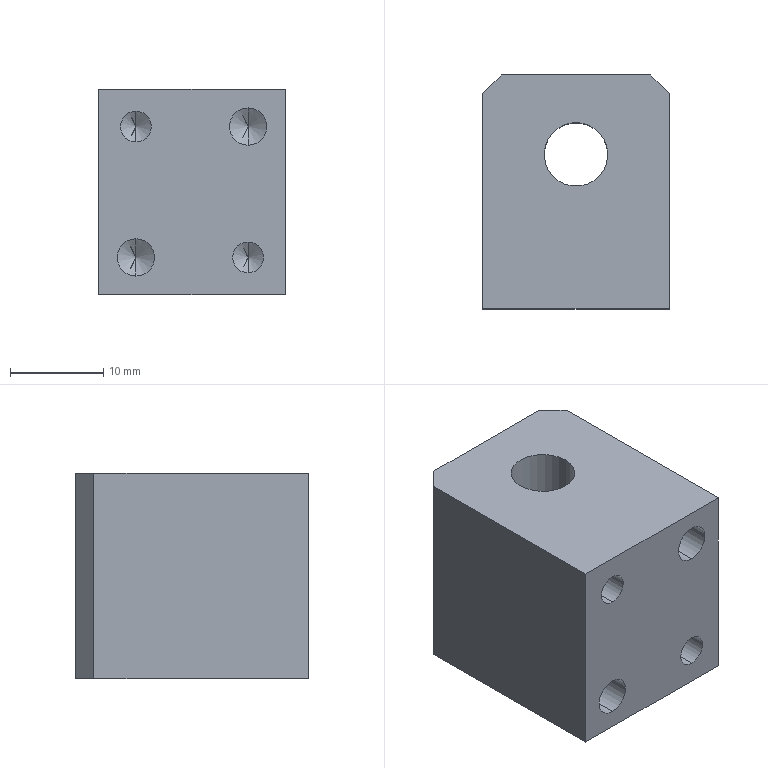Part | SolidWorks | features HoleWzd 3, Chamfer 1, Extrusion 1 | 1 solid | 26 faces | box 20 x 25 x 22 mm | volume 9700 mm3 | cylinder 10 | cone 8 | plane 8 | commonest cylinder face diameters 3.3 x4 4 x4 6.8 x2
STEP:
#1=CARTESIAN_POINT('',(6.,-4.5,9.));
#2=VERTEX_POINT('',#1);
#3=CARTESIAN_POINT('',(6.,-4.5,5.));
#4=VERTEX_POINT('',#3);
#5=CARTESIAN_POINT('',(6.,-4.5,7.));
#6=DIRECTION('',(0.,-1.,0.));
#7=DIRECTION('',(0.,0.,-1.));
#8=AXIS2_PLACEMENT_3D('',#5,#6,#7);
#9=CIRCLE('',#8,2.);
#10=EDGE_CURVE('',#2,#4,#9,.T.);
#11=ORIENTED_EDGE('',*,*,#10,.F.);
#12=CARTESIAN_POINT('',(6.,-12.5,9.));
#13=VERTEX_POINT('',#12);
#14=CARTESIAN_POINT('',(6.,-12.5,9.));
#15=DIRECTION('',(0.,-1.,0.));
#16=VECTOR('',#15,1000.);
#17=LINE('',#14,#16);
#18=EDGE_CURVE('',#2,#13,#17,.T.);
#19=ORIENTED_EDGE('',*,*,#18,.T.);
#20=CARTESIAN_POINT('',(6.,-12.5,5.));
#21=VERTEX_POINT('',#20);
#22=CARTESIAN_POINT('',(6.,-12.5,7.));
#23=DIRECTION('',(0.,-1.,0.));
#24=DIRECTION('',(0.,0.,-1.));
#25=AXIS2_PLACEMENT_3D('',#22,#23,#24);
#26=CIRCLE('',#25,2.);
#27=EDGE_CURVE('',#13,#21,#26,.T.);
#28=ORIENTED_EDGE('',*,*,#27,.T.);
#29=CARTESIAN_POINT('',(6.,-12.5,5.));
#30=DIRECTION('',(0.,-1.,0.));
#31=VECTOR('',#30,1000.);
#32=LINE('',#29,#31);
#33=EDGE_CURVE('',#4,#21,#32,.T.);
#34=ORIENTED_EDGE('',*,*,#33,.F.);
#35=EDGE_LOOP('',(#11,#19,#28,#34));
#36=FACE_OUTER_BOUND('',#35,.T.);
#37=CARTESIAN_POINT('',(6.,-12.5,7.));
#38=DIRECTION('',(0.,-1.,0.));
#39=DIRECTION('',(0.,0.,-1.));
#40=AXIS2_PLACEMENT_3D('',#37,#38,#39);
#41=CYLINDRICAL_SURFACE('',#40,2.);
#42=ADVANCED_FACE('',(#36),#41,.F.);
#43=CARTESIAN_POINT('',(6.,-3.298,7.));
#44=VERTEX_POINT('',#43);
#45=CARTESIAN_POINT('',(6.,-4.5,5.));
#46=DIRECTION('',(0.,-0.515,-0.8572));
#47=VECTOR('',#46,1000.);
#48=LINE('',#45,#47);
#49=EDGE_CURVE('',#44,#4,#48,.T.);
#50=ORIENTED_EDGE('',*,*,#49,.F.);
#51=CARTESIAN_POINT('',(6.,-4.5,9.));
#52=DIRECTION('',(0.,-0.515,0.8572));
#53=VECTOR('',#52,1000.);
#54=LINE('',#51,#53);
#55=EDGE_CURVE('',#44,#2,#54,.T.);
#56=ORIENTED_EDGE('',*,*,#55,.T.);
#57=ORIENTED_EDGE('',*,*,#10,.T.);
#58=EDGE_LOOP('',(#50,#56,#57));
#59=FACE_OUTER_BOUND('',#58,.T.);
#60=CARTESIAN_POINT('',(6.,-4.5,7.));
#61=DIRECTION('',(0.,-1.,0.));
#62=DIRECTION('',(0.,0.,-1.));
#63=AXIS2_PLACEMENT_3D('',#60,#61,#62);
#64=CONICAL_SURFACE('',#63,2.,1.03);
#65=ADVANCED_FACE('',(#59),#64,.F.);
#66=CARTESIAN_POINT('',(-6.,-4.5,-5.));
#67=VERTEX_POINT('',#66);
#68=CARTESIAN_POINT('',(-6.,-4.5,-9.));
#69=VERTEX_POINT('',#68);
#70=CARTESIAN_POINT('',(-6.,-4.5,-7.));
#71=DIRECTION('',(0.,-1.,0.));
#72=DIRECTION('',(0.,0.,-1.));
#73=AXIS2_PLACEMENT_3D('',#70,#71,#72);
#74=CIRCLE('',#73,2.);
#75=EDGE_CURVE('',#67,#69,#74,.T.);
#76=ORIENTED_EDGE('',*,*,#75,.F.);
#77=CARTESIAN_POINT('',(-6.,-12.5,-5.));
#78=VERTEX_POINT('',#77);
#79=CARTESIAN_POINT('',(-6.,-12.5,-5.));
#80=DIRECTION('',(0.,-1.,0.));
#81=VECTOR('',#80,1000.);
#82=LINE('',#79,#81);
#83=EDGE_CURVE('',#67,#78,#82,.T.);
#84=ORIENTED_EDGE('',*,*,#83,.T.);
#85=CARTESIAN_POINT('',(-6.,-12.5,-9.));
#86=VERTEX_POINT('',#85);
#87=CARTESIAN_POINT('',(-6.,-12.5,-7.));
#88=DIRECTION('',(0.,-1.,0.));
#89=DIRECTION('',(0.,0.,-1.));
#90=AXIS2_PLACEMENT_3D('',#87,#88,#89);
#91=CIRCLE('',#90,2.);
#92=EDGE_CURVE('',#78,#86,#91,.T.);
#93=ORIENTED_EDGE('',*,*,#92,.T.);
#94=CARTESIAN_POINT('',(-6.,-12.5,-9.));
#95=DIRECTION('',(0.,-1.,0.));
#96=VECTOR('',#95,1000.);
#97=LINE('',#94,#96);
#98=EDGE_CURVE('',#69,#86,#97,.T.);
#99=ORIENTED_EDGE('',*,*,#98,.F.);
#100=EDGE_LOOP('',(#76,#84,#93,#99));
#101=FACE_OUTER_BOUND('',#100,.T.);
#102=CARTESIAN_POINT('',(-6.,-12.5,-7.));
#103=DIRECTION('',(0.,-1.,0.));
#104=DIRECTION('',(0.,0.,-1.));
#105=AXIS2_PLACEMENT_3D('',#102,#103,#104);
#106=CYLINDRICAL_SURFACE('',#105,2.);
#107=ADVANCED_FACE('',(#101),#106,.F.);
#108=CARTESIAN_POINT('',(-6.,-3.298,-7.));
#109=VERTEX_POINT('',#108);
#110=CARTESIAN_POINT('',(-6.,-4.5,-9.));
#111=DIRECTION('',(0.,-0.515,-0.8572));
#112=VECTOR('',#111,1000.);
#113=LINE('',#110,#112);
#114=EDGE_CURVE('',#109,#69,#113,.T.);
#115=ORIENTED_EDGE('',*,*,#114,.F.);
#116=CARTESIAN_POINT('',(-6.,-4.5,-5.));
#117=DIRECTION('',(0.,-0.515,0.8572));
#118=VECTOR('',#117,1000.);
#119=LINE('',#116,#118);
#120=EDGE_CURVE('',#109,#67,#119,.T.);
#121=ORIENTED_EDGE('',*,*,#120,.T.);
#122=ORIENTED_EDGE('',*,*,#75,.T.);
#123=EDGE_LOOP('',(#115,#121,#122));
#124=FACE_OUTER_BOUND('',#123,.T.);
#125=CARTESIAN_POINT('',(-6.,-4.5,-7.));
#126=DIRECTION('',(0.,-1.,0.));
#127=DIRECTION('',(0.,0.,-1.));
#128=AXIS2_PLACEMENT_3D('',#125,#126,#127);
#129=CONICAL_SURFACE('',#128,2.,1.03);
#130=ADVANCED_FACE('',(#124),#129,.F.);
#131=CARTESIAN_POINT('',(-6.,-1.,8.65));
#132=VERTEX_POINT('',#131);
#133=CARTESIAN_POINT('',(-6.,-1.,5.35));
#134=VERTEX_POINT('',#133);
#135=CARTESIAN_POINT('',(-6.,-1.,7.));
#136=DIRECTION('',(0.,-1.,0.));
#137=DIRECTION('',(0.,0.,-1.));
#138=AXIS2_PLACEMENT_3D('',#135,#136,#137);
#139=CIRCLE('',#138,1.65);
#140=EDGE_CURVE('',#132,#134,#139,.T.);
#141=ORIENTED_EDGE('',*,*,#140,.F.);
#142=CARTESIAN_POINT('',(-6.,-12.5,8.65));
#143=VERTEX_POINT('',#142);
#144=CARTESIAN_POINT('',(-6.,-12.5,8.65));
#145=DIRECTION('',(0.,-1.,0.));
#146=VECTOR('',#145,1000.);
#147=LINE('',#144,#146);
#148=EDGE_CURVE('',#132,#143,#147,.T.);
#149=ORIENTED_EDGE('',*,*,#148,.T.);
#150=CARTESIAN_POINT('',(-6.,-12.5,5.35));
#151=VERTEX_POINT('',#150);
#152=CARTESIAN_POINT('',(-6.,-12.5,7.));
#153=DIRECTION('',(0.,-1.,0.));
#154=DIRECTION('',(0.,0.,-1.));
#155=AXIS2_PLACEMENT_3D('',#152,#153,#154);
#156=CIRCLE('',#155,1.65);
#157=EDGE_CURVE('',#143,#151,#156,.T.);
#158=ORIENTED_EDGE('',*,*,#157,.T.);
#159=CARTESIAN_POINT('',(-6.,-12.5,5.35));
#160=DIRECTION('',(0.,-1.,0.));
#161=VECTOR('',#160,1000.);
#162=LINE('',#159,#161);
#163=EDGE_CURVE('',#134,#151,#162,.T.);
#164=ORIENTED_EDGE('',*,*,#163,.F.);
#165=EDGE_LOOP('',(#141,#149,#158,#164));
#166=FACE_OUTER_BOUND('',#165,.T.);
#167=CARTESIAN_POINT('',(-6.,-12.5,7.));
#168=DIRECTION('',(0.,-1.,0.));
#169=DIRECTION('',(0.,0.,-1.));
#170=AXIS2_PLACEMENT_3D('',#167,#168,#169);
#171=CYLINDRICAL_SURFACE('',#170,1.65);
#172=ADVANCED_FACE('',(#166),#171,.F.);
#173=CARTESIAN_POINT('',(-6.,-0.00858,7.));
#174=VERTEX_POINT('',#173);
#175=CARTESIAN_POINT('',(-6.,-1.,5.35));
#176=DIRECTION('',(0.,-0.515,-0.8572));
#177=VECTOR('',#176,1000.);
#178=LINE('',#175,#177);
#179=EDGE_CURVE('',#174,#134,#178,.T.);
#180=ORIENTED_EDGE('',*,*,#179,.F.);
#181=CARTESIAN_POINT('',(-6.,-1.,8.65));
#182=DIRECTION('',(0.,-0.515,0.8572));
#183=VECTOR('',#182,1000.);
#184=LINE('',#181,#183);
#185=EDGE_CURVE('',#174,#132,#184,.T.);
#186=ORIENTED_EDGE('',*,*,#185,.T.);
#187=ORIENTED_EDGE('',*,*,#140,.T.);
#188=EDGE_LOOP('',(#180,#186,#187));
#189=FACE_OUTER_BOUND('',#188,.T.);
#190=CARTESIAN_POINT('',(-6.,-1.,7.));
#191=DIRECTION('',(0.,-1.,0.));
#192=DIRECTION('',(0.,0.,-1.));
#193=AXIS2_PLACEMENT_3D('',#190,#191,#192);
#194=CONICAL_SURFACE('',#193,1.65,1.03);
#195=ADVANCED_FACE('',(#189),#194,.F.);
#196=CARTESIAN_POINT('',(6.,-1.,-5.35));
#197=VERTEX_POINT('',#196);
#198=CARTESIAN_POINT('',(6.,-1.,-8.65));
#199=VERTEX_POINT('',#198);
#200=CARTESIAN_POINT('',(6.,-1.,-7.));
#201=DIRECTION('',(0.,-1.,0.));
#202=DIRECTION('',(0.,0.,-1.));
#203=AXIS2_PLACEMENT_3D('',#200,#201,#202);
#204=CIRCLE('',#203,1.65);
#205=EDGE_CURVE('',#197,#199,#204,.T.);
#206=ORIENTED_EDGE('',*,*,#205,.F.);
#207=CARTESIAN_POINT('',(6.,-12.5,-5.35));
#208=VERTEX_POINT('',#207);
#209=CARTESIAN_POINT('',(6.,-12.5,-5.35));
#210=DIRECTION('',(0.,-1.,0.));
#211=VECTOR('',#210,1000.);
#212=LINE('',#209,#211);
#213=EDGE_CURVE('',#197,#208,#212,.T.);
#214=ORIENTED_EDGE('',*,*,#213,.T.);
#215=CARTESIAN_POINT('',(6.,-12.5,-8.65));
#216=VERTEX_POINT('',#215);
#217=CARTESIAN_POINT('',(6.,-12.5,-7.));
#218=DIRECTION('',(0.,-1.,0.));
#219=DIRECTION('',(0.,0.,-1.));
#220=AXIS2_PLACEMENT_3D('',#217,#218,#219);
#221=CIRCLE('',#220,1.65);
#222=EDGE_CURVE('',#208,#216,#221,.T.);
#223=ORIENTED_EDGE('',*,*,#222,.T.);
#224=CARTESIAN_POINT('',(6.,-12.5,-8.65));
#225=DIRECTION('',(0.,-1.,0.));
#226=VECTOR('',#225,1000.);
#227=LINE('',#224,#226);
#228=EDGE_CURVE('',#199,#216,#227,.T.);
#229=ORIENTED_EDGE('',*,*,#228,.F.);
#230=EDGE_LOOP('',(#206,#214,#223,#229));
#231=FACE_OUTER_BOUND('',#230,.T.);
#232=CARTESIAN_POINT('',(6.,-12.5,-7.));
#233=DIRECTION('',(0.,-1.,0.));
#234=DIRECTION('',(0.,0.,-1.));
#235=AXIS2_PLACEMENT_3D('',#232,#233,#234);
#236=CYLINDRICAL_SURFACE('',#235,1.65);
#237=ADVANCED_FACE('',(#231),#236,.F.);
#238=CARTESIAN_POINT('',(6.,-0.00858,-7.));
#239=VERTEX_POINT('',#238);
#240=CARTESIAN_POINT('',(6.,-1.,-8.65));
#241=DIRECTION('',(0.,-0.515,-0.8572));
#242=VECTOR('',#241,1000.);
#243=LINE('',#240,#242);
#244=EDGE_CURVE('',#239,#199,#243,.T.);
#245=ORIENTED_EDGE('',*,*,#244,.F.);
#246=CARTESIAN_POINT('',(6.,-1.,-5.35));
#247=DIRECTION('',(0.,-0.515,0.8572));
#248=VECTOR('',#247,1000.);
#249=LINE('',#246,#248);
#250=EDGE_CURVE('',#239,#197,#249,.T.);
#251=ORIENTED_EDGE('',*,*,#250,.T.);
#252=ORIENTED_EDGE('',*,*,#205,.T.);
#253=EDGE_LOOP('',(#245,#251,#252));
#254=FACE_OUTER_BOUND('',#253,.T.);
#255=CARTESIAN_POINT('',(6.,-1.,-7.));
#256=DIRECTION('',(0.,-1.,0.));
#257=DIRECTION('',(0.,0.,-1.));
#258=AXIS2_PLACEMENT_3D('',#255,#256,#257);
#259=CONICAL_SURFACE('',#258,1.65,1.03);
#260=ADVANCED_FACE('',(#254),#259,.F.);
#261=CARTESIAN_POINT('',(-3.4,4.,-11.));
#262=VERTEX_POINT('',#261);
#263=CARTESIAN_POINT('',(3.4,4.,-11.));
#264=VERTEX_POINT('',#263);
#265=CARTESIAN_POINT('',(0.,4.,-11.));
#266=DIRECTION('',(0.,0.,1.));
#267=DIRECTION('',(1.,0.,0.));
#268=AXIS2_PLACEMENT_3D('',#265,#266,#267);
#269=CIRCLE('',#268,3.4);
#270=EDGE_CURVE('',#262,#264,#269,.T.);
#271=ORIENTED_EDGE('',*,*,#270,.F.);
#272=CARTESIAN_POINT('',(-3.4,4.,11.));
#273=VERTEX_POINT('',#272);
#274=CARTESIAN_POINT('',(-3.4,4.,11.));
#275=DIRECTION('',(0.,0.,1.));
#276=VECTOR('',#275,1000.);
#277=LINE('',#274,#276);
#278=EDGE_CURVE('',#262,#273,#277,.T.);
#279=ORIENTED_EDGE('',*,*,#278,.T.);
#280=CARTESIAN_POINT('',(3.4,4.,11.));
#281=VERTEX_POINT('',#280);
#282=CARTESIAN_POINT('',(0.,4.,11.));
#283=DIRECTION('',(0.,0.,1.));
#284=DIRECTION('',(1.,0.,0.));
#285=AXIS2_PLACEMENT_3D('',#282,#283,#284);
#286=CIRCLE('',#285,3.4);
#287=EDGE_CURVE('',#273,#281,#286,.T.);
#288=ORIENTED_EDGE('',*,*,#287,.T.);
#289=CARTESIAN_POINT('',(3.4,4.,11.));
#290=DIRECTION('',(0.,0.,1.));
#291=VECTOR('',#290,1000.);
#292=LINE('',#289,#291);
#293=EDGE_CURVE('',#264,#281,#292,.T.);
#294=ORIENTED_EDGE('',*,*,#293,.F.);
#295=EDGE_LOOP('',(#271,#279,#288,#294));
#296=FACE_OUTER_BOUND('',#295,.T.);
#297=CARTESIAN_POINT('',(0.,4.,11.));
#298=DIRECTION('',(0.,0.,1.));
#299=DIRECTION('',(1.,0.,0.));
#300=AXIS2_PLACEMENT_3D('',#297,#298,#299);
#301=CYLINDRICAL_SURFACE('',#300,3.4);
#302=ADVANCED_FACE('',(#296),#301,.F.);
#303=CARTESIAN_POINT('',(10.,-12.5,-11.));
#304=VERTEX_POINT('',#303);
#305=CARTESIAN_POINT('',(10.,10.5,-11.));
#306=VERTEX_POINT('',#305);
#307=CARTESIAN_POINT('',(10.,12.5,-11.));
#308=DIRECTION('',(0.,1.,0.));
#309=VECTOR('',#308,1000.);
#310=LINE('',#307,#309);
#311=EDGE_CURVE('',#304,#306,#310,.T.);
#312=ORIENTED_EDGE('',*,*,#311,.T.);
#313=CARTESIAN_POINT('',(10.,10.5,11.));
#314=VERTEX_POINT('',#313);
#315=CARTESIAN_POINT('',(10.,10.5,11.));
#316=DIRECTION('',(0.,0.,1.));
#317=VECTOR('',#316,1000.);
#318=LINE('',#315,#317);
#319=EDGE_CURVE('',#306,#314,#318,.T.);
#320=ORIENTED_EDGE('',*,*,#319,.T.);
#321=CARTESIAN_POINT('',(10.,-12.5,11.));
#322=VERTEX_POINT('',#321);
#323=CARTESIAN_POINT('',(10.,12.5,11.));
#324=DIRECTION('',(0.,1.,0.));
#325=VECTOR('',#324,1000.);
#326=LINE('',#323,#325);
#327=EDGE_CURVE('',#322,#314,#326,.T.);
#328=ORIENTED_EDGE('',*,*,#327,.F.);
#329=CARTESIAN_POINT('',(10.,-12.5,11.));
#330=DIRECTION('',(0.,0.,-1.));
#331=VECTOR('',#330,1000.);
#332=LINE('',#329,#331);
#333=EDGE_CURVE('',#322,#304,#332,.T.);
#334=ORIENTED_EDGE('',*,*,#333,.T.);
#335=EDGE_LOOP('',(#312,#320,#328,#334));
#336=FACE_OUTER_BOUND('',#335,.T.);
#337=CARTESIAN_POINT('',(10.,12.5,11.));
#338=DIRECTION('',(-1.,0.,0.));
#339=DIRECTION('',(0.,-1.,0.));
#340=AXIS2_PLACEMENT_3D('',#337,#338,#339);
#341=PLANE('',#340);
#342=ADVANCED_FACE('',(#336),#341,.F.);
#343=CARTESIAN_POINT('',(8.,12.5,11.));
#344=VERTEX_POINT('',#343);
#345=CARTESIAN_POINT('',(-8.,12.5,11.));
#346=VERTEX_POINT('',#345);
#347=CARTESIAN_POINT('',(-10.,12.5,11.));
#348=DIRECTION('',(-1.,0.,0.));
#349=VECTOR('',#348,1000.);
#350=LINE('',#347,#349);
#351=EDGE_CURVE('',#344,#346,#350,.T.);
#352=ORIENTED_EDGE('',*,*,#351,.F.);
#353=CARTESIAN_POINT('',(8.,12.5,-11.));
#354=VERTEX_POINT('',#353);
#355=CARTESIAN_POINT('',(8.,12.5,11.));
#356=DIRECTION('',(0.,0.,-1.));
#357=VECTOR('',#356,1000.);
#358=LINE('',#355,#357);
#359=EDGE_CURVE('',#344,#354,#358,.T.);
#360=ORIENTED_EDGE('',*,*,#359,.T.);
#361=CARTESIAN_POINT('',(-8.,12.5,-11.));
#362=VERTEX_POINT('',#361);
#363=CARTESIAN_POINT('',(-10.,12.5,-11.));
#364=DIRECTION('',(-1.,0.,0.));
#365=VECTOR('',#364,1000.);
#366=LINE('',#363,#365);
#367=EDGE_CURVE('',#354,#362,#366,.T.);
#368=ORIENTED_EDGE('',*,*,#367,.T.);
#369=CARTESIAN_POINT('',(-8.,12.5,11.));
#370=DIRECTION('',(0.,0.,1.));
#371=VECTOR('',#370,1000.);
#372=LINE('',#369,#371);
#373=EDGE_CURVE('',#362,#346,#372,.T.);
#374=ORIENTED_EDGE('',*,*,#373,.T.);
#375=EDGE_LOOP('',(#352,#360,#368,#374));
#376=FACE_OUTER_BOUND('',#375,.T.);
#377=CARTESIAN_POINT('',(-10.,12.5,11.));
#378=DIRECTION('',(0.,-1.,0.));
#379=DIRECTION('',(0.,0.,-1.));
#380=AXIS2_PLACEMENT_3D('',#377,#378,#379);
#381=PLANE('',#380);
#382=ADVANCED_FACE('',(#376),#381,.F.);
#383=CARTESIAN_POINT('',(-10.,10.5,11.));
#384=VERTEX_POINT('',#383);
#385=CARTESIAN_POINT('',(-10.,-12.5,11.));
#386=VERTEX_POINT('',#385);
#387=CARTESIAN_POINT('',(-10.,12.5,11.));
#388=DIRECTION('',(0.,-1.,0.));
#389=VECTOR('',#388,1000.);
#390=LINE('',#387,#389);
#391=EDGE_CURVE('',#384,#386,#390,.T.);
#392=ORIENTED_EDGE('',*,*,#391,.F.);
#393=CARTESIAN_POINT('',(-10.,10.5,-11.));
#394=VERTEX_POINT('',#393);
#395=CARTESIAN_POINT('',(-10.,10.5,11.));
#396=DIRECTION('',(0.,0.,-1.));
#397=VECTOR('',#396,1000.);
#398=LINE('',#395,#397);
#399=EDGE_CURVE('',#384,#394,#398,.T.);
#400=ORIENTED_EDGE('',*,*,#399,.T.);
#401=CARTESIAN_POINT('',(-10.,-12.5,-11.));
#402=VERTEX_POINT('',#401);
#403=CARTESIAN_POINT('',(-10.,12.5,-11.));
#404=DIRECTION('',(0.,-1.,0.));
#405=VECTOR('',#404,1000.);
#406=LINE('',#403,#405);
#407=EDGE_CURVE('',#394,#402,#406,.T.);
#408=ORIENTED_EDGE('',*,*,#407,.T.);
#409=CARTESIAN_POINT('',(-10.,-12.5,11.));
#410=DIRECTION('',(0.,0.,-1.));
#411=VECTOR('',#410,1000.);
#412=LINE('',#409,#411);
#413=EDGE_CURVE('',#386,#402,#412,.T.);
#414=ORIENTED_EDGE('',*,*,#413,.F.);
#415=EDGE_LOOP('',(#392,#400,#408,#414));
#416=FACE_OUTER_BOUND('',#415,.T.);
#417=CARTESIAN_POINT('',(-10.,12.5,11.));
#418=DIRECTION('',(1.,0.,0.));
#419=DIRECTION('',(0.,1.,0.));
#420=AXIS2_PLACEMENT_3D('',#417,#418,#419);
#421=PLANE('',#420);
#422=ADVANCED_FACE('',(#416),#421,.F.);
#423=CARTESIAN_POINT('',(6.,-12.5,7.));
#424=DIRECTION('',(0.,-1.,0.));
#425=DIRECTION('',(0.,0.,-1.));
#426=AXIS2_PLACEMENT_3D('',#423,#424,#425);
#427=CIRCLE('',#426,2.);
#428=EDGE_CURVE('',#21,#13,#427,.T.);
#429=ORIENTED_EDGE('',*,*,#428,.F.);
#430=ORIENTED_EDGE('',*,*,#27,.F.);
#431=EDGE_LOOP('',(#429,#430));
#432=FACE_BOUND('',#431,.T.);
#433=CARTESIAN_POINT('',(-6.,-12.5,-7.));
#434=DIRECTION('',(0.,-1.,0.));
#435=DIRECTION('',(0.,0.,-1.));
#436=AXIS2_PLACEMENT_3D('',#433,#434,#435);
#437=CIRCLE('',#436,2.);
#438=EDGE_CURVE('',#86,#78,#437,.T.);
#439=ORIENTED_EDGE('',*,*,#438,.F.);
#440=ORIENTED_EDGE('',*,*,#92,.F.);
#441=EDGE_LOOP('',(#439,#440));
#442=FACE_BOUND('',#441,.T.);
#443=CARTESIAN_POINT('',(-6.,-12.5,7.));
#444=DIRECTION('',(0.,-1.,0.));
#445=DIRECTION('',(0.,0.,-1.));
#446=AXIS2_PLACEMENT_3D('',#443,#444,#445);
#447=CIRCLE('',#446,1.65);
#448=EDGE_CURVE('',#151,#143,#447,.T.);
#449=ORIENTED_EDGE('',*,*,#448,.F.);
#450=ORIENTED_EDGE('',*,*,#157,.F.);
#451=EDGE_LOOP('',(#449,#450));
#452=FACE_BOUND('',#451,.T.);
#453=CARTESIAN_POINT('',(6.,-12.5,-7.));
#454=DIRECTION('',(0.,-1.,0.));
#455=DIRECTION('',(0.,0.,-1.));
#456=AXIS2_PLACEMENT_3D('',#453,#454,#455);
#457=CIRCLE('',#456,1.65);
#458=EDGE_CURVE('',#216,#208,#457,.T.);
#459=ORIENTED_EDGE('',*,*,#458,.F.);
#460=ORIENTED_EDGE('',*,*,#222,.F.);
#461=EDGE_LOOP('',(#459,#460));
#462=FACE_BOUND('',#461,.T.);
#463=CARTESIAN_POINT('',(-10.,-12.5,-11.));
#464=DIRECTION('',(1.,0.,0.));
#465=VECTOR('',#464,1000.);
#466=LINE('',#463,#465);
#467=EDGE_CURVE('',#402,#304,#466,.T.);
#468=ORIENTED_EDGE('',*,*,#467,.T.);
#469=ORIENTED_EDGE('',*,*,#333,.F.);
#470=CARTESIAN_POINT('',(-10.,-12.5,11.));
#471=DIRECTION('',(1.,0.,0.));
#472=VECTOR('',#471,1000.);
#473=LINE('',#470,#472);
#474=EDGE_CURVE('',#386,#322,#473,.T.);
#475=ORIENTED_EDGE('',*,*,#474,.F.);
#476=ORIENTED_EDGE('',*,*,#413,.T.);
#477=EDGE_LOOP('',(#468,#469,#475,#476));
#478=FACE_OUTER_BOUND('',#477,.T.);
#479=CARTESIAN_POINT('',(-10.,-12.5,11.));
#480=DIRECTION('',(0.,1.,0.));
#481=DIRECTION('',(0.,0.,1.));
#482=AXIS2_PLACEMENT_3D('',#479,#480,#481);
#483=PLANE('',#482);
#484=ADVANCED_FACE('',(#432,#442,#452,#462,#478),#483,.F.);
#485=CARTESIAN_POINT('',(0.,4.,11.));
#486=DIRECTION('',(0.,0.,1.));
#487=DIRECTION('',(1.,0.,0.));
#488=AXIS2_PLACEMENT_3D('',#485,#486,#487);
#489=CIRCLE('',#488,3.4);
#490=EDGE_CURVE('',#281,#273,#489,.T.);
#491=ORIENTED_EDGE('',*,*,#490,.F.);
#492=ORIENTED_EDGE('',*,*,#287,.F.);
#493=EDGE_LOOP('',(#491,#492));
#494=FACE_BOUND('',#493,.T.);
#495=ORIENTED_EDGE('',*,*,#327,.T.);
#496=CARTESIAN_POINT('',(10.25,10.25,11.));
#497=DIRECTION('',(-0.7071,0.7071,0.));
#498=VECTOR('',#497,1000.);
#499=LINE('',#496,#498);
#500=EDGE_CURVE('',#314,#344,#499,.T.);
#501=ORIENTED_EDGE('',*,*,#500,.T.);
#502=ORIENTED_EDGE('',*,*,#351,.T.);
#503=CARTESIAN_POINT('',(-10.25,10.25,11.));
#504=DIRECTION('',(-0.7071,-0.7071,0.));
#505=VECTOR('',#504,1000.);
#506=LINE('',#503,#505);
#507=EDGE_CURVE('',#346,#384,#506,.T.);
#508=ORIENTED_EDGE('',*,*,#507,.T.);
#509=ORIENTED_EDGE('',*,*,#391,.T.);
#510=ORIENTED_EDGE('',*,*,#474,.T.);
#511=EDGE_LOOP('',(#495,#501,#502,#508,#509,#510));
#512=FACE_OUTER_BOUND('',#511,.T.);
#513=CARTESIAN_POINT('',(0.,0.,11.));
#514=DIRECTION('',(0.,0.,1.));
#515=DIRECTION('',(1.,0.,0.));
#516=AXIS2_PLACEMENT_3D('',#513,#514,#515);
#517=PLANE('',#516);
#518=ADVANCED_FACE('',(#494,#512),#517,.T.);
#519=CARTESIAN_POINT('',(0.,4.,-11.));
#520=DIRECTION('',(0.,0.,1.));
#521=DIRECTION('',(1.,0.,0.));
#522=AXIS2_PLACEMENT_3D('',#519,#520,#521);
#523=CIRCLE('',#522,3.4);
#524=EDGE_CURVE('',#264,#262,#523,.T.);
#525=ORIENTED_EDGE('',*,*,#524,.T.);
#526=ORIENTED_EDGE('',*,*,#270,.T.);
#527=EDGE_LOOP('',(#525,#526));
#528=FACE_BOUND('',#527,.T.);
#529=ORIENTED_EDGE('',*,*,#367,.F.);
#530=CARTESIAN_POINT('',(8.,12.5,-11.));
#531=DIRECTION('',(0.7071,-0.7071,0.));
#532=VECTOR('',#531,1000.);
#533=LINE('',#530,#532);
#534=EDGE_CURVE('',#354,#306,#533,.T.);
#535=ORIENTED_EDGE('',*,*,#534,.T.);
#536=ORIENTED_EDGE('',*,*,#311,.F.);
#537=ORIENTED_EDGE('',*,*,#467,.F.);
#538=ORIENTED_EDGE('',*,*,#407,.F.);
#539=CARTESIAN_POINT('',(-10.,10.5,-11.));
#540=DIRECTION('',(0.7071,0.7071,0.));
#541=VECTOR('',#540,1000.);
#542=LINE('',#539,#541);
#543=EDGE_CURVE('',#394,#362,#542,.T.);
#544=ORIENTED_EDGE('',*,*,#543,.T.);
#545=EDGE_LOOP('',(#529,#535,#536,#537,#538,#544));
#546=FACE_OUTER_BOUND('',#545,.T.);
#547=CARTESIAN_POINT('',(0.,0.,-11.));
#548=DIRECTION('',(0.,0.,1.));
#549=DIRECTION('',(1.,0.,0.));
#550=AXIS2_PLACEMENT_3D('',#547,#548,#549);
#551=PLANE('',#550);
#552=ADVANCED_FACE('',(#528,#546),#551,.F.);
#553=ORIENTED_EDGE('',*,*,#500,.F.);
#554=ORIENTED_EDGE('',*,*,#319,.F.);
#555=ORIENTED_EDGE('',*,*,#534,.F.);
#556=ORIENTED_EDGE('',*,*,#359,.F.);
#557=EDGE_LOOP('',(#553,#554,#555,#556));
#558=FACE_OUTER_BOUND('',#557,.T.);
#559=CARTESIAN_POINT('',(8.,12.5,11.));
#560=DIRECTION('',(-0.7071,-0.7071,0.));
#561=DIRECTION('',(0.,0.,-1.));
#562=AXIS2_PLACEMENT_3D('',#559,#560,#561);
#563=PLANE('',#562);
#564=ADVANCED_FACE('',(#558),#563,.F.);
#565=ORIENTED_EDGE('',*,*,#507,.F.);
#566=ORIENTED_EDGE('',*,*,#373,.F.);
#567=ORIENTED_EDGE('',*,*,#543,.F.);
#568=ORIENTED_EDGE('',*,*,#399,.F.);
#569=EDGE_LOOP('',(#565,#566,#567,#568));
#570=FACE_OUTER_BOUND('',#569,.T.);
#571=CARTESIAN_POINT('',(-10.,10.5,11.));
#572=DIRECTION('',(0.7071,-0.7071,0.));
#573=DIRECTION('',(0.,0.,-1.));
#574=AXIS2_PLACEMENT_3D('',#571,#572,#573);
#575=PLANE('',#574);
#576=ADVANCED_FACE('',(#570),#575,.F.);
#577=ORIENTED_EDGE('',*,*,#278,.F.);
#578=ORIENTED_EDGE('',*,*,#524,.F.);
#579=ORIENTED_EDGE('',*,*,#293,.T.);
#580=ORIENTED_EDGE('',*,*,#490,.T.);
#581=EDGE_LOOP('',(#577,#578,#579,#580));
#582=FACE_OUTER_BOUND('',#581,.T.);
#583=CARTESIAN_POINT('',(0.,4.,11.));
#584=DIRECTION('',(0.,0.,1.));
#585=DIRECTION('',(1.,0.,0.));
#586=AXIS2_PLACEMENT_3D('',#583,#584,#585);
#587=CYLINDRICAL_SURFACE('',#586,3.4);
#588=ADVANCED_FACE('',(#582),#587,.F.);
#589=ORIENTED_EDGE('',*,*,#250,.F.);
#590=ORIENTED_EDGE('',*,*,#244,.T.);
#591=CARTESIAN_POINT('',(6.,-1.,-7.));
#592=DIRECTION('',(0.,-1.,0.));
#593=DIRECTION('',(0.,0.,-1.));
#594=AXIS2_PLACEMENT_3D('',#591,#592,#593);
#595=CIRCLE('',#594,1.65);
#596=EDGE_CURVE('',#199,#197,#595,.T.);
#597=ORIENTED_EDGE('',*,*,#596,.T.);
#598=EDGE_LOOP('',(#589,#590,#597));
#599=FACE_OUTER_BOUND('',#598,.T.);
#600=CARTESIAN_POINT('',(6.,-1.,-7.));
#601=DIRECTION('',(0.,-1.,0.));
#602=DIRECTION('',(0.,0.,-1.));
#603=AXIS2_PLACEMENT_3D('',#600,#601,#602);
#604=CONICAL_SURFACE('',#603,1.65,1.03);
#605=ADVANCED_FACE('',(#599),#604,.F.);
#606=ORIENTED_EDGE('',*,*,#213,.F.);
#607=ORIENTED_EDGE('',*,*,#596,.F.);
#608=ORIENTED_EDGE('',*,*,#228,.T.);
#609=ORIENTED_EDGE('',*,*,#458,.T.);
#610=EDGE_LOOP('',(#606,#607,#608,#609));
#611=FACE_OUTER_BOUND('',#610,.T.);
#612=CARTESIAN_POINT('',(6.,-12.5,-7.));
#613=DIRECTION('',(0.,-1.,0.));
#614=DIRECTION('',(0.,0.,-1.));
#615=AXIS2_PLACEMENT_3D('',#612,#613,#614);
#616=CYLINDRICAL_SURFACE('',#615,1.65);
#617=ADVANCED_FACE('',(#611),#616,.F.);
#618=ORIENTED_EDGE('',*,*,#185,.F.);
#619=ORIENTED_EDGE('',*,*,#179,.T.);
#620=CARTESIAN_POINT('',(-6.,-1.,7.));
#621=DIRECTION('',(0.,-1.,0.));
#622=DIRECTION('',(0.,0.,-1.));
#623=AXIS2_PLACEMENT_3D('',#620,#621,#622);
#624=CIRCLE('',#623,1.65);
#625=EDGE_CURVE('',#134,#132,#624,.T.);
#626=ORIENTED_EDGE('',*,*,#625,.T.);
#627=EDGE_LOOP('',(#618,#619,#626));
#628=FACE_OUTER_BOUND('',#627,.T.);
#629=CARTESIAN_POINT('',(-6.,-1.,7.));
#630=DIRECTION('',(0.,-1.,0.));
#631=DIRECTION('',(0.,0.,-1.));
#632=AXIS2_PLACEMENT_3D('',#629,#630,#631);
#633=CONICAL_SURFACE('',#632,1.65,1.03);
#634=ADVANCED_FACE('',(#628),#633,.F.);
#635=ORIENTED_EDGE('',*,*,#148,.F.);
#636=ORIENTED_EDGE('',*,*,#625,.F.);
#637=ORIENTED_EDGE('',*,*,#163,.T.);
#638=ORIENTED_EDGE('',*,*,#448,.T.);
#639=EDGE_LOOP('',(#635,#636,#637,#638));
#640=FACE_OUTER_BOUND('',#639,.T.);
#641=CARTESIAN_POINT('',(-6.,-12.5,7.));
#642=DIRECTION('',(0.,-1.,0.));
#643=DIRECTION('',(0.,0.,-1.));
#644=AXIS2_PLACEMENT_3D('',#641,#642,#643);
#645=CYLINDRICAL_SURFACE('',#644,1.65);
#646=ADVANCED_FACE('',(#640),#645,.F.);
#647=ORIENTED_EDGE('',*,*,#120,.F.);
#648=ORIENTED_EDGE('',*,*,#114,.T.);
#649=CARTESIAN_POINT('',(-6.,-4.5,-7.));
#650=DIRECTION('',(0.,-1.,0.));
#651=DIRECTION('',(0.,0.,-1.));
#652=AXIS2_PLACEMENT_3D('',#649,#650,#651);
#653=CIRCLE('',#652,2.);
#654=EDGE_CURVE('',#69,#67,#653,.T.);
#655=ORIENTED_EDGE('',*,*,#654,.T.);
#656=EDGE_LOOP('',(#647,#648,#655));
#657=FACE_OUTER_BOUND('',#656,.T.);
#658=CARTESIAN_POINT('',(-6.,-4.5,-7.));
#659=DIRECTION('',(0.,-1.,0.));
#660=DIRECTION('',(0.,0.,-1.));
#661=AXIS2_PLACEMENT_3D('',#658,#659,#660);
#662=CONICAL_SURFACE('',#661,2.,1.03);
#663=ADVANCED_FACE('',(#657),#662,.F.);
#664=ORIENTED_EDGE('',*,*,#83,.F.);
#665=ORIENTED_EDGE('',*,*,#654,.F.);
#666=ORIENTED_EDGE('',*,*,#98,.T.);
#667=ORIENTED_EDGE('',*,*,#438,.T.);
#668=EDGE_LOOP('',(#664,#665,#666,#667));
#669=FACE_OUTER_BOUND('',#668,.T.);
#670=CARTESIAN_POINT('',(-6.,-12.5,-7.));
#671=DIRECTION('',(0.,-1.,0.));
#672=DIRECTION('',(0.,0.,-1.));
#673=AXIS2_PLACEMENT_3D('',#670,#671,#672);
#674=CYLINDRICAL_SURFACE('',#673,2.);
#675=ADVANCED_FACE('',(#669),#674,.F.);
#676=ORIENTED_EDGE('',*,*,#55,.F.);
#677=ORIENTED_EDGE('',*,*,#49,.T.);
#678=CARTESIAN_POINT('',(6.,-4.5,7.));
#679=DIRECTION('',(0.,-1.,0.));
#680=DIRECTION('',(0.,0.,-1.));
#681=AXIS2_PLACEMENT_3D('',#678,#679,#680);
#682=CIRCLE('',#681,2.);
#683=EDGE_CURVE('',#4,#2,#682,.T.);
#684=ORIENTED_EDGE('',*,*,#683,.T.);
#685=EDGE_LOOP('',(#676,#677,#684));
#686=FACE_OUTER_BOUND('',#685,.T.);
#687=CARTESIAN_POINT('',(6.,-4.5,7.));
#688=DIRECTION('',(0.,-1.,0.));
#689=DIRECTION('',(0.,0.,-1.));
#690=AXIS2_PLACEMENT_3D('',#687,#688,#689);
#691=CONICAL_SURFACE('',#690,2.,1.03);
#692=ADVANCED_FACE('',(#686),#691,.F.);
#693=ORIENTED_EDGE('',*,*,#18,.F.);
#694=ORIENTED_EDGE('',*,*,#683,.F.);
#695=ORIENTED_EDGE('',*,*,#33,.T.);
#696=ORIENTED_EDGE('',*,*,#428,.T.);
#697=EDGE_LOOP('',(#693,#694,#695,#696));
#698=FACE_OUTER_BOUND('',#697,.T.);
#699=CARTESIAN_POINT('',(6.,-12.5,7.));
#700=DIRECTION('',(0.,-1.,0.));
#701=DIRECTION('',(0.,0.,-1.));
#702=AXIS2_PLACEMENT_3D('',#699,#700,#701);
#703=CYLINDRICAL_SURFACE('',#702,2.);
#704=ADVANCED_FACE('',(#698),#703,.F.);
#705=CLOSED_SHELL('',(#42,#65,#107,#130,#172,#195,#237,#260,#302,#342,#382,#422,#484,#518,#552,#564,#576,#588,#605,#617,#634,#646,#663,#675,#692,#704));
#706=MANIFOLD_SOLID_BREP('',#705);
#707=CARTESIAN_POINT('',(0.,0.,0.));
#708=DIRECTION('',(0.,0.,1.));
#709=DIRECTION('',(1.,0.,0.));
#710=AXIS2_PLACEMENT_3D('',#707,#708,#709);
#711=(LENGTH_UNIT()NAMED_UNIT(*)SI_UNIT(.MILLI.,.METRE.));
#712=UNCERTAINTY_MEASURE_WITH_UNIT(LENGTH_MEASURE(0.00001),#711,'','');
#713=(NAMED_UNIT(*)PLANE_ANGLE_UNIT()SI_UNIT($,.RADIAN.));
#714=(NAMED_UNIT(*)SI_UNIT($,.STERADIAN.)SOLID_ANGLE_UNIT());
#715=(GEOMETRIC_REPRESENTATION_CONTEXT(3)GLOBAL_UNCERTAINTY_ASSIGNED_CONTEXT((#712))GLOBAL_UNIT_ASSIGNED_CONTEXT((#711,#713,#714))REPRESENTATION_CONTEXT('',''));
#716=ADVANCED_BREP_SHAPE_REPRESENTATION('',(#706,#710),#715);